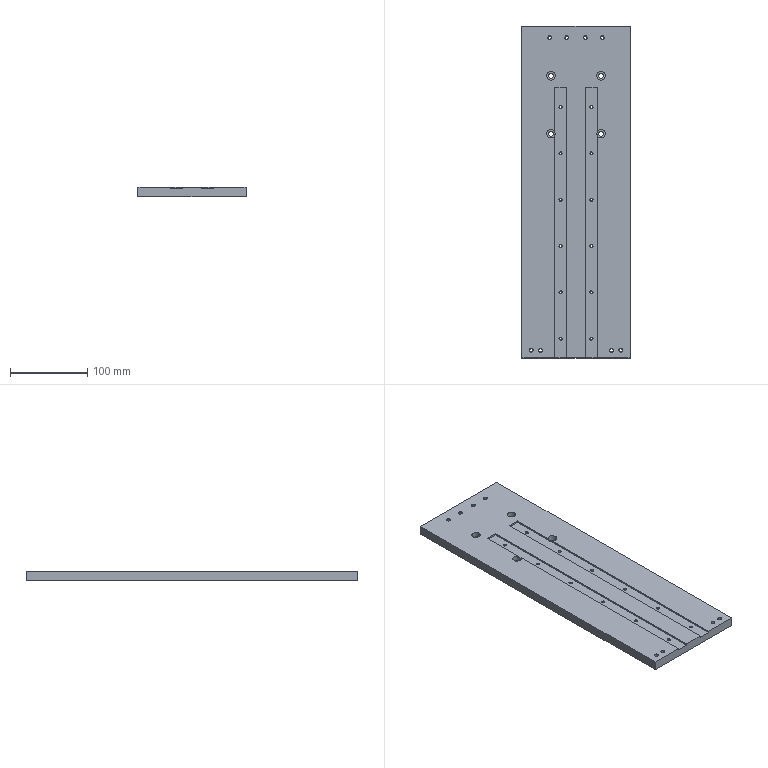Part | SolidWorks | features BaseBody 1, Fillet 1, HoleWzd 1, ICE 1 | 1 solid | 122 faces | box 140 x 430 x 12 mm | volume 670240 mm3 | cylinder 58 | cone 40 | plane 24 | commonest cylinder face diameters 3.3 x24 4.2 x16 6.6 x8 11 x8 6 x2